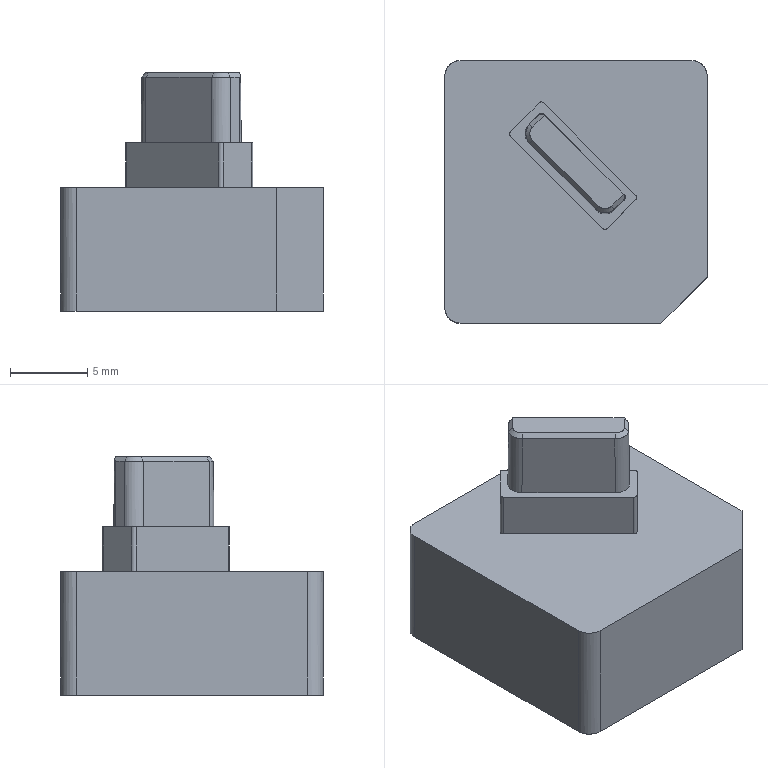NC program | PowerMill | posted with a generic post | part box 17 x 17 x 15.424 mm
Lines 3247 to 4312 of 24748:
N3344 M6
N3345 S18000 M03
N3346 G00 G90 X0.0 Y0.0
N3347 G43 Z10.804 H14
N3348
N3349 G05 P10000 R8
N3350 X1.6082 Y4.7339
N3351 Z0.794
N3352 G01 Z-0.406 F1200.0
N3353 X1.5606 Y4.6806 F2000.0
N3354 X1.5193 Y4.6224
N3355 X1.4846 Y4.5599
N3356 X1.4572 Y4.4939
N3357 X1.4373 Y4.4253
N3358 X1.4251 Y4.3549
N3359 X1.4209 Y4.2836
N3360 X1.4247 Y4.2122
N3361 X1.4363 Y4.1418
N3362 X1.4558 Y4.073
N3363 X1.4828 Y4.0068
N3364 X1.517 Y3.9441
N3365 X1.558 Y3.8856
N3366 X1.6053 Y3.832
N3367 X1.6085 Y3.8288
N3368 X1.7494 Y3.688
N3369 X2.1047 Y3.3323
N3370 X2.4605 Y2.9769
N3371 X3.1826 Y2.2539
N3372 X3.4605 Y1.977
N3373 X3.7378 Y1.6995
N3374 X3.8898 Y1.5451
N3375 X4.0697 Y1.3685
N3376 X4.1747 Y1.2654
N3377 X4.3095 Y1.1279
N3378 X4.4178 Y1.0089
N3379 X4.4892 Y0.9237
N3380 X4.5558 Y0.8347
N3381 X4.6169 Y0.7398
N3382 X4.6724 Y0.6391
N3383 X4.7218 Y0.5327
N3384 X4.7651 Y0.4211
N3385 X4.8017 Y0.3045
N3386 X4.83 Y0.1893
N3387 X4.8506 Y0.0727
N3388 X4.8634 Y-0.045
N3389 X4.8684 Y-0.1635
N3390 X4.8654 Y-0.2822
N3391 X4.8545 Y-0.4008
N3392 X4.8356 Y-0.5187
N3393 X4.8089 Y-0.6353
N3394 X4.7743 Y-0.7501
N3395 X4.7322 Y-0.8625
N3396 X4.6826 Y-0.9719
N3397 X4.626 Y-1.0778
N3398 X4.5624 Y-1.1796
N3399 X4.4923 Y-1.2771
N3400 X4.4158 Y-1.3697
N3401 X4.3335 Y-1.4572
N3402 X4.2476 Y-1.542
N3403 X3.857 Y-1.9321
N3404 X3.5858 Y-2.2036
N3405 X3.4823 Y-2.301
N3406 X3.3746 Y-2.3916
N3407 X3.2629 Y-2.4752
N3408 X3.1477 Y-2.5516
N3409 X3.0293 Y-2.6206
N3410 X2.9081 Y-2.6822
N3411 X2.7835 Y-2.7367
N3412 X2.6531 Y-2.7853
N3413 X2.5213 Y-2.8259
N3414 X2.3985 Y-2.8564
N3415 X2.2612 Y-2.8826
N3416 X2.1233 Y-2.9007
N3417 X1.9851 Y-2.9109
N3418 X1.847 Y-2.9131
N3419 X1.7088 Y-2.9074
N3420 X1.5711 Y-2.8936
N3421 X1.4344 Y-2.872
N3422 X1.2994 Y-2.8425
N3423 X1.1664 Y-2.8053
N3424 X1.0358 Y-2.7605
N3425 X0.9081 Y-2.7083
N3426 X0.7837 Y-2.649
N3427 X0.6609 Y-2.5821
N3428 X0.5442 Y-2.5096
N3429 X0.4336 Y-2.4318
N3430 X0.3376 Y-2.3557
N3431 X0.2437 Y-2.2724
N3432 X0.1308 Y-2.1629
N3433 X-0.0749 Y-1.9571
N3434 X-1.3805 Y-0.6516
N3435 X-3.5829 Y1.5506
N3436 X-4.0378 Y2.0056
N3437 X-4.1367 Y2.1062
N3438 X-4.2297 Y2.2114
N3439 X-4.3162 Y2.3212
N3440 X-4.396 Y2.4353
N3441 X-4.4689 Y2.5535
N3442 X-4.5347 Y2.6753
N3443 X-4.5933 Y2.8005
N3444 X-4.6445 Y2.9287
N3445 X-4.6881 Y3.0596
N3446 X-4.7241 Y3.1928
N3447 X-4.7524 Y3.328
N3448 X-4.773 Y3.4648
N3449 X-4.7857 Y3.603
N3450 X-4.7906 Y3.7414
N3451 X-4.7876 Y3.8795
N3452 X-4.7768 Y4.0171
N3453 X-4.758 Y4.1538
N3454 X-4.7314 Y4.2892
N3455 X-4.697 Y4.423
N3456 X-4.6549 Y4.5547
N3457 X-4.6052 Y4.6838
N3458 X-4.548 Y4.8102
N3459 X-4.4836 Y4.9331
N3460 X-4.4122 Y5.0523
N3461 X-4.3339 Y5.1674
N3462 X-4.249 Y5.2781
N3463 X-4.1578 Y5.3839
N3464 X-4.0605 Y5.4849
N3465 X-3.5634 Y5.9813
N3466 X-3.3467 Y6.1994
N3467 X-3.2565 Y6.2851
N3468 X-3.1621 Y6.3638
N3469 X-3.064 Y6.4354
N3470 X-2.9625 Y6.4997
N3471 X-2.858 Y6.5566
N3472 X-2.7505 Y6.6062
N3473 X-2.6399 Y6.6485
N3474 X-2.5266 Y6.6833
N3475 X-2.4111 Y6.7107
N3476 X-2.2939 Y6.7302
N3477 X-2.1753 Y6.742
N3478 X-2.0558 Y6.7458
N3479 X-1.9361 Y6.7417
N3480 X-1.8167 Y6.7296
N3481 X-1.698 Y6.7095
N3482 X-1.5807 Y6.6816
N3483 X-1.4655 Y6.6459
N3484 X-1.3528 Y6.6027
N3485 X-1.2432 Y6.5522
N3486 X-1.137 Y6.4946
N3487 X-1.0599 Y6.4468
N3488 X-0.9887 Y6.3962
N3489 X-0.9208 Y6.3415
N3490 X-0.8478 Y6.2777
N3491 X-0.7663 Y6.2019
N3492 X-0.6736 Y6.1117
N3493 X-0.5647 Y6.0027
N3494 X-0.4285 Y5.8654
N3495 X-0.3645 Y5.8013
N3496 X0.0232 Y5.4136
N3497 X0.4112 Y5.0263
N3498 X1.3049 Y4.1322
N3499 X1.6085 Y3.8288
N3500 X1.6617 Y3.7812
N3501 X1.72 Y3.7398
N3502 X1.7825 Y3.7052
N3503 X1.8485 Y3.6777
N3504 X1.9171 Y3.6578
N3505 X1.9875 Y3.6457
N3506 X2.0588 Y3.6415
N3507 X2.1301 Y3.6452
N3508 X2.2006 Y3.6569
N3509 X2.2694 Y3.6764
N3510 X2.3355 Y3.7034
N3511 X2.3983 Y3.7376
N3512 X2.4568 Y3.7786
N3513 X2.5103 Y3.8258
N3514 X2.5136 Y3.8291
N3515 X1.6086 Y4.734 Z-0.426
N3516 X1.561 Y4.6808
N3517 X1.5196 Y4.6226
N3518 X1.485 Y4.5601
N3519 X1.4575 Y4.4941
N3520 X1.4376 Y4.4255
N3521 X1.4254 Y4.3551
N3522 X1.4212 Y4.2838
N3523 X1.4249 Y4.2124
N3524 X1.4366 Y4.1419
N3525 X1.456 Y4.0732
N3526 X1.483 Y4.007
N3527 X1.5172 Y3.9443
N3528 X1.5582 Y3.8858
N3529 X1.6054 Y3.8322
N3530 X1.6086 Y3.8289
N3531 X1.7034 Y3.7341
N3532 X3.1654 Y2.2722
N3533 X4.3253 Y1.1117
N3534 X4.4129 Y1.0183
N3535 X4.4933 Y0.9212
N3536 X4.5663 Y0.8208
N3537 X4.6319 Y0.7172
N3538 X4.6891 Y0.6125
N3539 X4.7392 Y0.5044
N3540 X4.7819 Y0.3931
N3541 X4.8171 Y0.2793
N3542 X4.8447 Y0.1633
N3543 X4.8645 Y0.0455
N3544 X4.8764 Y-0.0736
N3545 X4.8804 Y-0.1933
N3546 X4.8764 Y-0.3132
N3547 X4.8644 Y-0.4324
N3548 X4.8445 Y-0.5505
N3549 X4.8169 Y-0.6669
N3550 X4.7817 Y-0.7811
N3551 X4.739 Y-0.8925
N3552 X4.689 Y-1.0008
N3553 X4.6343 Y-1.1016
N3554 X4.5723 Y-1.1993
N3555 X4.5021 Y-1.2956
N3556 X4.4231 Y-1.3903
N3557 X4.3353 Y-1.4835
N3558 X4.2405 Y-1.5774
N3559 X3.7611 Y-2.0567
N3560 X3.6142 Y-2.2038
N3561 X3.5119 Y-2.3013
N3562 X3.4052 Y-2.3928
N3563 X3.2962 Y-2.4764
N3564 X3.185 Y-2.5518
N3565 X3.0717 Y-2.6197
N3566 X2.9544 Y-2.6818
N3567 X2.828 Y-2.7399
N3568 X2.6983 Y-2.7907
N3569 X2.5657 Y-2.8341
N3570 X2.484 Y-2.8567
N3571 X2.4027 Y-2.8752
N3572 X2.3561 Y-2.8859
N3573 X2.2219 Y-2.9087
N3574 X2.0826 Y-2.9246
N3575 X1.9515 Y-2.9323
N3576 X1.8203 Y-2.9326
N3577 X1.6805 Y-2.9252
N3578 X1.5419 Y-2.9098
N3579 X1.4049 Y-2.8866
N3580 X1.2699 Y-2.8556
N3581 X1.1375 Y-2.8171
N3582 X1.0076 Y-2.7711
N3583 X0.8774 Y-2.7166
N3584 X0.7512 Y-2.6552
N3585 X0.6296 Y-2.5872
N3586 X0.5128 Y-2.5129
N3587 X0.4012 Y-2.4324
N3588 X0.3077 Y-2.357
N3589 X0.2162 Y-2.2744
N3590 X0.1018 Y-2.1623
N3591 X-0.2422 Y-1.8183
N3592 X-3.3461 Y1.2858
N3593 X-4.0838 Y2.0235
N3594 X-4.18 Y2.1239
N3595 X-4.2702 Y2.2292
N3596 X-4.3542 Y2.3392
N3597 X-4.4319 Y2.4539
N3598 X-4.5028 Y2.5728
N3599 X-4.567 Y2.6956
N3600 X-4.624 Y2.8221
N3601 X-4.6737 Y2.9517
N3602 X-4.716 Y3.0841
N3603 X-4.7507 Y3.2188
N3604 X-4.7776 Y3.3555
N3605 X-4.7967 Y3.4935
N3606 X-4.8078 Y3.6324
N3607 X-4.8109 Y3.7716
N3608 X-4.806 Y3.9106
N3609 X-4.7933 Y4.049
N3610 X-4.7726 Y4.1862
N3611 X-4.7441 Y4.322
N3612 X-4.708 Y4.4559
N3613 X-4.6643 Y4.5874
N3614 X-4.6133 Y4.7161
N3615 X-4.5549 Y4.8416
N3616 X-4.4894 Y4.9638
N3617 X-4.4167 Y5.0824
N3618 X-4.337 Y5.1971
N3619 X-4.2505 Y5.3076
N3620 X-4.1573 Y5.4137
N3621 X-4.0583 Y5.5154
N3622 X-3.7646 Y5.8078
N3623 X-3.5421 Y6.031
N3624 X-3.4533 Y6.1222
N3625 X-3.3602 Y6.2152
N3626 X-3.2654 Y6.3024
N3627 X-3.1692 Y6.3821
N3628 X-3.0725 Y6.4529
N3629 X-2.975 Y6.5148
N3630 X-2.8765 Y6.5684
N3631 X-2.7764 Y6.6145
N3632 X-2.6743 Y6.6538
N3633 X-2.5699 Y6.6871
N3634 X-2.4614 Y6.7151
N3635 X-2.3448 Y6.7373
N3636 X-2.2271 Y6.7516
N3637 X-2.1085 Y6.758
N3638 X-1.9895 Y6.7565
N3639 X-1.8706 Y6.7471
N3640 X-1.7523 Y6.7296
N3641 X-1.6353 Y6.7043
N3642 X-1.52 Y6.6712
N3643 X-1.4071 Y6.6305
N3644 X-1.2971 Y6.5823
N3645 X-1.1905 Y6.527
N3646 X-1.0876 Y6.4647
N3647 X-0.9908 Y6.397
N3648 X-0.8943 Y6.3201
N3649 X-0.7953 Y6.2314
N3650 X-0.6911 Y6.1286
N3651 X0.0252 Y5.4123
N3652 X1.6086 Y3.8289
N3653 X1.6619 Y3.7813
N3654 X1.7201 Y3.7399
N3655 X1.7826 Y3.7053
N3656 X1.8486 Y3.6778
N3657 X1.9172 Y3.6579
N3658 X1.9876 Y3.6457
N3659 X2.0589 Y3.6415
N3660 X2.1302 Y3.6452
N3661 X2.2007 Y3.6569
N3662 X2.2694 Y3.6763
N3663 X2.3356 Y3.7033
N3664 X2.3984 Y3.7375
N3665 X2.4569 Y3.7785
N3666 X2.5105 Y3.8257
N3667 X2.5137 Y3.8289
N3668 X1.6088 Y4.7341 Z-0.446
N3669 X1.5611 Y4.6809
N3670 X1.5198 Y4.6227
N3671 X1.4851 Y4.5602
N3672 X1.4576 Y4.4942
N3673 X1.4377 Y4.4256
N3674 X1.4255 Y4.3552
N3675 X1.4213 Y4.2839
N3676 X1.425 Y4.2125
N3677 X1.4367 Y4.1421
N3678 X1.4561 Y4.0733
N3679 X1.4831 Y4.0071
N3680 X1.5173 Y3.9444
N3681 X1.5583 Y3.8859
N3682 X1.6055 Y3.8323
N3683 X1.6087 Y3.8291
N3684 X2.0613 Y3.3764
N3685 X4.1939 Y1.244
N3686 X4.3256 Y1.1122
N3687 X4.4086 Y1.024
N3688 X4.4869 Y0.9299
N3689 X4.5609 Y0.8286
N3690 X4.6298 Y0.7212
N3691 X4.6883 Y0.6175
N3692 X4.7399 Y0.5102
N3693 X4.7841 Y0.3997
N3694 X4.821 Y0.2865
N3695 X4.8502 Y0.1709
N3696 X4.8717 Y0.0533
N3697 X4.8853 Y-0.0657
N3698 X4.891 Y-0.1855
N3699 X4.8887 Y-0.3054
N3700 X4.8785 Y-0.4249
N3701 X4.8603 Y-0.5435
N3702 X4.8343 Y-0.6607
N3703 X4.8017 Y-0.7729
N3704 X4.7617 Y-0.8824
N3705 X4.7142 Y-0.9896
N3706 X4.6592 Y-1.0942
N3707 X4.5966 Y-1.1962
N3708 X4.5264 Y-1.2955
N3709 X4.4485 Y-1.3918
N3710 X4.3629 Y-1.4851
N3711 X4.2708 Y-1.576
N3712 X3.9386 Y-1.9067
N3713 X3.6429 Y-2.2042
N3714 X3.5336 Y-2.3086
N3715 X3.423 Y-2.4037
N3716 X3.311 Y-2.49
N3717 X3.1978 Y-2.5675
N3718 X3.0833 Y-2.6366
N3719 X2.9671 Y-2.6978
N3720 X2.835 Y-2.7584
N3721 X2.7066 Y-2.8091
N3722 X2.5809 Y-2.8507
N3723 X2.5601 Y-2.8568
N3724 X2.4254 Y-2.8915
N3725 X2.4067 Y-2.8952
N3726 X2.2878 Y-2.9187
N3727 X2.1481 Y-2.9381
N3728 X2.0076 Y-2.9496
N3729 X1.8672 Y-2.9532
N3730 X1.7279 Y-2.9488
N3731 X1.5906 Y-2.9365
N3732 X1.4547 Y-2.9165
N3733 X1.3183 Y-2.8883
N3734 X1.1828 Y-2.8522
N3735 X1.0491 Y-2.8083
N3736 X0.9185 Y-2.757
N3737 X0.7916 Y-2.6986
N3738 X0.6693 Y-2.6337
N3739 X0.5522 Y-2.5626
N3740 X0.4588 Y-2.499
N3741 X0.3682 Y-2.4316
N3742 X0.2811 Y-2.3598
N3743 X0.1975 Y-2.2838
N3744 X0.1164 Y-2.205
N3745 X0.0365 Y-2.1252
N3746 X-1.7839 Y-0.3048
N3747 X-3.5094 Y1.4207
N3748 X-4.0256 Y1.9372
N3749 X-4.1284 Y2.0408
N3750 X-4.2228 Y2.1419
N3751 X-4.3112 Y2.2484
N3752 X-4.3937 Y2.3601
N3753 X-4.4698 Y2.4766
N3754 X-4.5393 Y2.5976
N3755 X-4.6019 Y2.7227
N3756 X-4.6572 Y2.8511
N3757 X-4.7055 Y2.9833
N3758 X-4.7461 Y3.1176
N3759 X-4.7788 Y3.2536
N3760 X-4.8037 Y3.3909
N3761 X-4.8206 Y3.529
N3762 X-4.8296 Y3.6678
N3763 X-4.8306 Y3.8067
N3764 X-4.8236 Y3.9454
N3765 X-4.8088 Y4.0837
N3766 X-4.786 Y4.2225
N3767 X-4.7554 Y4.3593
N3768 X-4.7172 Y4.4939
N3769 X-4.6715 Y4.6258
N3770 X-4.6184 Y4.7546
N3771 X-4.558 Y4.8801
N3772 X-4.4906 Y5.0018
N3773 X-4.4163 Y5.1195
N3774 X-4.3353 Y5.2329
N3775 X-4.2478 Y5.3417
N3776 X-4.1541 Y5.4456
N3777 X-4.0557 Y5.5461
N3778 X-3.7666 Y5.8346
N3779 X-3.5192 Y6.0827
N3780 X-3.4392 Y6.1642
N3781 X-3.3578 Y6.2444
N3782 X-3.2691 Y6.3259
N3783 X-3.1772 Y6.4018
N3784 X-3.0898 Y6.4651
N3785 X-3.005 Y6.5186
N3786 X-2.9195 Y6.5658
N3787 X-2.8314 Y6.6083
N3788 X-2.741 Y6.6464
N3789 X-2.6281 Y6.6861
N3790 X-2.5126 Y6.7183
N3791 X-2.3952 Y6.7428
N3792 X-2.2764 Y6.7594
N3793 X-2.1569 Y6.768
N3794 X-2.0374 Y6.7687
N3795 X-1.9185 Y6.7614
N3796 X-1.8008 Y6.7462
N3797 X-1.6848 Y6.7233
N3798 X-1.571 Y6.6927
N3799 X-1.4596 Y6.6545
N3800 X-1.3677 Y6.6166
N3801 X-1.2804 Y6.5757
N3802 X-1.1951 Y6.5308
N3803 X-1.1106 Y6.4807
N3804 X-1.0251 Y6.4231
N3805 X-0.9359 Y6.355
N3806 X-0.8393 Y6.2719
N3807 X-0.7449 Y6.1828
N3808 X-0.6599 Y6.0984
N3809 X-0.58 Y6.0174
N3810 X-0.502 Y5.9386
N3811 X-0.4241 Y5.861
N3812 X-0.3431 Y5.7812
N3813 X-0.0454 Y5.4831
N3814 X0.268 Y5.1701
N3815 X0.7299 Y4.7077
N3816 X1.1885 Y4.2493
N3817 X1.6087 Y3.8291
N3818 X1.662 Y3.7814
N3819 X1.7202 Y3.7401
N3820 X1.7827 Y3.7054
N3821 X1.8487 Y3.6779
N3822 X1.9173 Y3.658
N3823 X1.9877 Y3.6458
N3824 X2.059 Y3.6416
N3825 X2.1303 Y3.6453
N3826 X2.2008 Y3.657
N3827 X2.2696 Y3.6764
N3828 X2.3358 Y3.7034
N3829 X2.3985 Y3.7376
N3830 X2.457 Y3.7786
N3831 X2.5106 Y3.8258
N3832 X2.5138 Y3.829
N3833 X1.6088 Y4.7343 Z-0.466
N3834 X1.5612 Y4.681
N3835 X1.5198 Y4.6228
N3836 X1.4852 Y4.5603
N3837 X1.4577 Y4.4943
N3838 X1.4378 Y4.4257
N3839 X1.4256 Y4.3553
N3840 X1.4214 Y4.284
N3841 X1.4251 Y4.2126
N3842 X1.4368 Y4.1422
N3843 X1.4562 Y4.0734
N3844 X1.4832 Y4.0072
N3845 X1.5174 Y3.9445
N3846 X1.5584 Y3.886
N3847 X1.6056 Y3.8324
N3848 X1.6088 Y3.8292
N3849 X2.0042 Y3.4339
N3850 X3.2344 Y2.2035
N3851 X4.3256 Y1.1125
N3852 X4.4075 Y1.0257
N3853 X4.485 Y0.9333
N3854 X4.558 Y0.8343
N3855 X4.6262 Y0.7283
N3856 X4.6884 Y0.6181
N3857 X4.7412 Y0.5113
N3858 X4.787 Y0.4014
N3859 X4.8253 Y0.2886
N3860 X4.856 Y0.1735
N3861 X4.879 Y0.0563
N3862 X4.8941 Y-0.0623
N3863 X4.9013 Y-0.1817
N3864 X4.9005 Y-0.3012
N3865 X4.8917 Y-0.4203
N3866 X4.8751 Y-0.5383
N3867 X4.8506 Y-0.6549
N3868 X4.8184 Y-0.7696
N3869 X4.7789 Y-0.8819
N3870 X4.7318 Y-0.9927
N3871 X4.6787 Y-1.0979
N3872 X4.6199 Y-1.197
N3873 X4.556 Y-1.2898
N3874 X4.487 Y-1.3761
N3875 X4.413 Y-1.458
N3876 X4.3319 Y-1.5427
N3877 X4.2496 Y-1.6263
N3878 X4.1622 Y-1.7138
N3879 X4.0383 Y-1.8366
N3880 X3.9548 Y-1.919
N3881 X3.8713 Y-2.0016
N3882 X3.7881 Y-2.0844
N3883 X3.7056 Y-2.1678
N3884 X3.6234 Y-2.2517
N3885 X3.5186 Y-2.3498
N3886 X3.4097 Y-2.4408
N3887 X3.2974 Y-2.5245
N3888 X3.1807 Y-2.6017
N3889 X3.0591 Y-2.6725
N3890 X2.934 Y-2.7362
N3891 X2.806 Y-2.7925
N3892 X2.6754 Y-2.8412
N3893 X2.6286 Y-2.8565
N3894 X2.4933 Y-2.8954
N3895 X2.411 Y-2.9141
N3896 X2.3561 Y-2.9266
N3897 X2.2176 Y-2.9499
N3898 X2.0781 Y-2.9652
N3899 X1.938 Y-2.9726
N3900 X1.7979 Y-2.972
N3901 X1.6582 Y-2.9634
N3902 X1.5193 Y-2.9469
N3903 X1.3815 Y-2.9225
N3904 X1.2452 Y-2.8903
N3905 X1.1107 Y-2.8504
N3906 X0.9781 Y-2.8028
N3907 X0.8483 Y-2.7476
N3908 X0.722 Y-2.6853
N3909 X0.5996 Y-2.616
N3910 X0.4813 Y-2.5399
N3911 X0.3798 Y-2.4666
N3912 X0.2803 Y-2.3855
N3913 X0.1735 Y-2.289
N3914 X0.0813 Y-2.199
N3915 X-1.4919 Y-0.6251
N3916 X-2.6883 Y0.5713
N3917 X-3.6907 Y1.5736
N3918 X-3.9949 Y1.8764
N3919 X-4.0877 Y1.9693
N3920 X-4.2017 Y2.0889
N3921 X-4.2928 Y2.1931
N3922 X-4.3727 Y2.2955
N3923 X-4.4479 Y2.4046
N3924 X-4.5197 Y2.5225
N3925 X-4.5882 Y2.6501
N3926 X-4.6465 Y2.7732
N3927 X-4.6978 Y2.9
N3928 X-4.7421 Y3.0307
N3929 X-4.7792 Y3.1649
N3930 X-4.8088 Y3.3021
N3931 X-4.8308 Y3.4412
N3932 X-4.8448 Y3.5808
N3933 X-4.8509 Y3.7208
N3934 X-4.849 Y3.8607
N3935 X-4.8391 Y4.0002
N3936 X-4.8212 Y4.1391
N3937 X-4.7954 Y4.2769
N3938 X-4.7618 Y4.4133
N3939 X-4.7204 Y4.5479
N3940 X-4.6713 Y4.6805
N3941 X-4.6153 Y4.809
N3942 X-4.5522 Y4.9338
N3943 X-4.4823 Y5.0545
N3944 X-4.4058 Y5.1706
N3945 X-4.3231 Y5.2817
N3946 X-4.2345 Y5.3875
N3947 X-4.1401 Y5.4879
N3948 X-3.8296 Y5.8006
N3949 X-3.6717 Y5.9561
N3950 X-3.5532 Y6.0759
N3951 X-3.421 Y6.2112
N3952 X-3.3213 Y6.3067
N3953 X-3.2327 Y6.3832
N3954 X-3.1454 Y6.4493
N3955 X-3.0451 Y6.5154
N3956 X-2.9411 Y6.5744
N3957 X-2.834 Y6.6261
N3958 X-2.7242 Y6.6703
N3959 X-2.6117 Y6.7071
N3960 X-2.4952 Y6.7369
N3961 X-2.3769 Y6.759
N3962 X-2.2575 Y6.7731
N3963 X-2.1375 Y6.7793
N3964 X-2.0177 Y6.7775
N3965 X-1.8987 Y6.7677
N3966 X-1.7809 Y6.7501
N3967 X-1.665 Y6.7248
N3968 X-1.5514 Y6.6918
N3969 X-1.4404 Y6.6513
N3970 X-1.3478 Y6.6108
N3971 X-1.2602 Y6.5673
N3972 X-1.1748 Y6.5202
N3973 X-1.0919 Y6.4693
N3974 X-1.0116 Y6.4142
N3975 X-0.9334 Y6.3544
N3976 X-0.8531 Y6.2862
N3977 X-0.7651 Y6.2041
N3978 X-0.6505 Y6.0894
N3979 X-0.5713 Y6.0094
N3980 X0.6244 Y4.8135
N3981 X1.6088 Y3.8292
N3982 X1.6621 Y3.7815
N3983 X1.7203 Y3.7402
N3984 X1.7828 Y3.7055
N3985 X1.8488 Y3.6781
N3986 X1.9174 Y3.6581
N3987 X1.9878 Y3.646
N3988 X2.0591 Y3.6417
N3989 X2.1305 Y3.6455
N3990 X2.2009 Y3.6571
N3991 X2.2697 Y3.6766
N3992 X2.3359 Y3.7036
N3993 X2.3986 Y3.7378
N3994 X2.4571 Y3.7788
N3995 X2.5107 Y3.826
N3996 X2.5139 Y3.8292
N3997 X1.609 Y4.7344 Z-0.486
N3998 X1.5614 Y4.6812
N3999 X1.52 Y4.6229
N4000 X1.4854 Y4.5605
N4001 X1.4579 Y4.4944
N4002 X1.4379 Y4.4258
N4003 X1.4258 Y4.3554
N4004 X1.4216 Y4.2841
N4005 X1.4253 Y4.2128
N4006 X1.4369 Y4.1423
N4007 X1.4564 Y4.0736
N4008 X1.4834 Y4.0074
N4009 X1.5176 Y3.9447
N4010 X1.5586 Y3.8861
N4011 X1.6058 Y3.8326
N4012 X1.609 Y3.8293
N4013 X1.9336 Y3.5047
N4014 X3.9286 Y1.51
N4015 X4.3256 Y1.1127
N4016 X4.4124 Y1.0202
N4017 X4.4935 Y0.922
N4018 X4.5688 Y0.8185
N4019 X4.6378 Y0.71
N4020 X4.7004 Y0.5968
N4021 X4.7561 Y0.4794
N4022 X4.8008 Y0.3689
N4023 X4.8382 Y0.2558
N4024 X4.868 Y0.1406
N4025 X4.8901 Y0.0236
N4026 X4.9043 Y-0.0946
N4027 X4.9106 Y-0.2137
N4028 X4.909 Y-0.3333
N4029 X4.8994 Y-0.4526
N4030 X4.8819 Y-0.5711
N4031 X4.8565 Y-0.6883
N4032 X4.8234 Y-0.8034
N4033 X4.7827 Y-0.9159
N4034 X4.7347 Y-1.0254
N4035 X4.6796 Y-1.1313
N4036 X4.6176 Y-1.2333
N4037 X4.5491 Y-1.3309
N4038 X4.4851 Y-1.4109
N4039 X4.4126 Y-1.4905
N4040 X4.3146 Y-1.588
N4041 X4.2022 Y-1.6981
N4042 X4.1 Y-1.8019
N4043 X3.8189 Y-2.0824
N4044 X3.6726 Y-2.2299
N4045 X3.5662 Y-2.3333
N4046 X3.4608 Y-2.4255
N4047 X3.3559 Y-2.5074
N4048 X3.2469 Y-2.5832
N4049 X3.126 Y-2.6578
N4050 X3.0018 Y-2.7252
N4051 X2.8749 Y-2.7851
N4052 X2.7458 Y-2.8372
N4053 X2.6921 Y-2.8564
N4054 X2.5575 Y-2.8986
N4055 X2.4208 Y-2.9332
N4056 X2.4149 Y-2.9344
N4057 X2.2823 Y-2.9601
N4058 X2.1425 Y-2.979
N4059 X2.0018 Y-2.9901
N4060 X1.8608 Y-2.9932
N4061 X1.7199 Y-2.9883
N4062 X1.5797 Y-2.9754
N4063 X1.4407 Y-2.9547
N4064 X1.3033 Y-2.9261
N4065 X1.168 Y-2.8899
N4066 X1.0351 Y-2.846
N4067 X0.9049 Y-2.7946
N4068 X0.7778 Y-2.7359
N4069 X0.688 Y-2.6889
N4070 X0.5999 Y-2.6388
N4071 X0.5139 Y-2.5858
N4072 X0.4301 Y-2.5294
N4073 X0.349 Y-2.4692
N4074 X0.2699 Y-2.4046
N4075 X0.1806 Y-2.3242
N4076 X0.0809 Y-2.2272
N4077 X0.001 Y-2.1467
N4078 X-0.0707 Y-2.0746
N4079 X-0.1456 Y-2.0
N4080 X-0.7117 Y-1.4333
N4081 X-1.2984 Y-0.8469
N4082 X-2.4609 Y0.3154
N4083 X-3.5327 Y1.3874
N4084 X-3.8994 Y1.7541
N4085 X-4.0233 Y1.8763
N4086 X-4.1526 Y2.0071
N4087 X-4.2596 Y2.1243
N4088 X-4.3507 Y2.2341
N4089 X-4.4292 Y2.3398
N4090 X-4.4975 Y2.4441
N4091 X-4.5691 Y2.5683
N4092 X-4.6335 Y2.6958
N4093 X-4.6903 Y2.8262
N4094 X-4.7396 Y2.9592
N4095 X-4.7812 Y3.0942
N4096 X-4.8149 Y3.2304
N4097 X-4.8408 Y3.3679
N4098 X-4.8588 Y3.5067
N4099 X-4.8689 Y3.6464
N4100 X-4.8711 Y3.7868
N4101 X-4.8652 Y3.9274
N4102 X-4.8514 Y4.068
N4103 X-4.8296 Y4.2083
N4104 X-4.8008 Y4.3437
N4105 X-4.764 Y4.4782
N4106 X-4.7193 Y4.612
N4107 X-4.6667 Y4.7437
N4108 X-4.6071 Y4.8718
N4109 X-4.541 Y4.9952
N4110 X-4.4759 Y5.1021
N4111 X-4.4056 Y5.2055
N4112 X-4.33 Y5.3051
N4113 X-4.2429 Y5.4081
N4114 X-4.1434 Y5.5151
N4115 X-4.0507 Y5.6086
N4116 X-3.9562 Y5.7016
N4117 X-3.7006 Y5.9575
N4118 X-3.4451 Y6.2137
N4119 X-3.3615 Y6.2961
N4120 X-3.2745 Y6.3742
N4121 X-3.1824 Y6.4463
N4122 X-3.0852 Y6.5124
N4123 X-2.9831 Y6.5721
N4124 X-2.8767 Y6.6251
N4125 X-2.7664 Y6.6711
N4126 X-2.6527 Y6.7099
N4127 X-2.5361 Y6.7412
N4128 X-2.4173 Y6.7649
N4129 X-2.3011 Y6.7803
N4130 X-2.1849 Y6.788
N4131 X-2.0684
N4132 X-1.9518 Y6.7803
N4133 X-1.8352 Y6.7648
N4134 X-1.7188 Y6.7414
N4135 X-1.603 Y6.71
N4136 X-1.4879 Y6.6707
N4137 X-1.3739 Y6.6233
N4138 X-1.2614 Y6.568
N4139 X-1.1508 Y6.5048
N4140 X-1.0425 Y6.4338
N4141 X-0.9372 Y6.3552
N4142 X-0.8352 Y6.2693
N4143 X-0.7374 Y6.1764
N4144 X-0.6414 Y6.0796
N4145 X-0.1617 Y5.6003
N4146 X0.3766 Y5.0617
N4147 X1.609 Y3.8293
N4148 X1.6623 Y3.7817
N4149 X1.7205 Y3.7403
N4150 X1.783 Y3.7057
N4151 X1.849 Y3.6782
N4152 X1.9176 Y3.6583
N4153 X1.988 Y3.6461
N4154 X2.0593 Y3.6419
N4155 X2.1306 Y3.6456
N4156 X2.2011 Y3.6573
N4157 X2.2698 Y3.6767
N4158 X2.336 Y3.7037
N4159 X2.3988 Y3.7379
N4160 X2.4573 Y3.7789
N4161 X2.5109 Y3.8261
N4162 X2.5141 Y3.8293
N4163 X1.6091 Y4.7345 Z-0.506
N4164 X1.5614 Y4.6813
N4165 X1.5201 Y4.623
N4166 X1.4854 Y4.5605
N4167 X1.4579 Y4.4945
N4168 X1.438 Y4.4259
N4169 X1.4259 Y4.3555
N4170 X1.4216 Y4.2842
N4171 X1.4254 Y4.2129
N4172 X1.437 Y4.1424
N4173 X1.4565 Y4.0737
N4174 X1.4835 Y4.0075
N4175 X1.5177 Y3.9447
N4176 X1.5587 Y3.8862
N4177 X1.6059 Y3.8327
N4178 X1.6091 Y3.8294
N4179 X2.2857 Y3.1529
N4180 X3.3982 Y2.0404
N4181 X4.1622 Y1.2761
N4182 X4.3062 Y1.1324
N4183 X4.4013 Y1.0323
N4184 X4.4741 Y0.9475
N4185 X4.5416 Y0.8584
N4186 X4.611 Y0.7541
N4187 X4.6753 Y0.6433
N4188 X4.7343 Y0.526
N4189 X4.7877 Y0.4022
N4190 X4.8283 Y0.2921
N4191 X4.8618 Y0.1797
N4192 X4.8877 Y0.0649
N4193 X4.9059 Y-0.0521
N4194 X4.9163 Y-0.1706
N4195 X4.9189 Y-0.2901
N4196 X4.9134 Y-0.41
N4197 X4.8999 Y-0.5298
N4198 X4.8785 Y-0.6486
N4199 X4.8502 Y-0.7627
N4200 X4.8143 Y-0.8749
N4201 X4.7706 Y-0.9853
N4202 X4.7192 Y-1.0935
N4203 X4.6603 Y-1.1988
N4204 X4.6022 Y-1.2885
N4205 X4.535 Y-1.378
N4206 X4.4558 Y-1.4708
N4207 X4.3612 Y-1.5701
N4208 X4.2457 Y-1.6841
N4209 X4.0349 Y-1.8967
N4210 X3.8508 Y-2.0797
N4211 X3.673 Y-2.2585
N4212 X3.5697 Y-2.3574
N4213 X3.4602 Y-2.4513
N4214 X3.3489 Y-2.5367
N4215 X3.2331 Y-2.616
N4216 X3.1127 Y-2.6887
N4217 X2.988 Y-2.7546
N4218 X2.8598 Y-2.8134
N4219 X2.7514 Y-2.8564
N4220 X2.6165 Y-2.9022
N4221 X2.4796 Y-2.9401
N4222 X2.419 Y-2.9533
N4223 X2.3414 Y-2.9702
N4224 X2.202 Y-2.9924
N4225 X2.0615 Y-3.0067
N4226 X1.9205 Y-3.013
N4227 X1.7793 Y-3.0114
N4228 X1.6384 Y-3.0018
N4229 X1.498 Y-2.9843
N4230 X1.3588 Y-2.9588
N4231 X1.2211 Y-2.9255
N4232 X1.0855 Y-2.8846
N4233 X0.9526 Y-2.836
N4234 X0.8227 Y-2.7802
N4235 X0.6964 Y-2.7171
N4236 X0.5739 Y-2.6471
N4237 X0.4556 Y-2.5703
N4238 X0.3417 Y-2.4869
N4239 X0.2328 Y-2.3972
N4240 X0.1288 Y-2.3017
N4241 X0.0013 Y-2.1754
N4242 X-0.1899 Y-1.9837
N4243 X-2.5486 Y0.375
N4244 X-3.5574 Y1.3835
N4245 X-3.8359 Y1.6623
N4246 X-3.8972 Y1.7236
N4247 X-3.9587 Y1.7847
N4248 X-4.0204 Y1.8458
N4249 X-4.0821 Y1.9068
N4250 X-4.1435 Y1.9682
N4251 X-4.2039 Y2.0304
N4252 X-4.2625 Y2.0942
N4253 X-4.3184 Y2.1602
N4254 X-4.3714 Y2.2286
N4255 X-4.4221 Y2.2987
N4256 X-4.4713 Y2.37
N4257 X-4.5442 Y2.4845
N4258 X-4.6108 Y2.604
N4259 X-4.671 Y2.7283
N4260 X-4.7246 Y2.8571
N4261 X-4.7712 Y2.99
N4262 X-4.8107 Y3.1267
N4263 X-4.8423 Y3.2644
N4264 X-4.8662 Y3.4038
N4265 X-4.8821 Y3.5443
N4266 X-4.8901 Y3.6854
N4267 Y3.8269
N4268 X-4.8822 Y3.9681
N4269 X-4.8662 Y4.1086
N4270 X-4.8424 Y4.248
N4271 X-4.8107 Y4.3858
N4272 X-4.7714 Y4.5213
N4273 X-4.7241 Y4.6556
N4274 X-4.6697 Y4.7866
N4275 X-4.6081 Y4.9138
N4276 X-4.5396 Y5.037
N4277 X-4.4644 Y5.156
N4278 X-4.3825 Y5.2705
N4279 X-4.2942 Y5.3803
N4280 X-4.1996 Y5.4852
N4281 X-4.1012 Y5.5848
N4282 X-3.4034 Y6.2834
N4283 X-3.319 Y6.3623
N4284 X-3.229 Y6.4354
N4285 X-3.1336 Y6.5028
N4286 X-3.033 Y6.5641
N4287 X-2.9277 Y6.6189
N4288 X-2.8182 Y6.667
N4289 X-2.705 Y6.7079
N4290 X-2.5886 Y6.7416
N4291 X-2.4698 Y6.7676
N4292 X-2.3543 Y6.785
N4293 X-2.2372 Y6.7947
N4294 X-2.1187 Y6.7965
N4295 X-1.9992 Y6.7904
N4296 X-1.8795 Y6.7763
N4297 X-1.7625 Y6.7546
N4298 X-1.6453 Y6.7247
N4299 X-1.5283 Y6.6867
N4300 X-1.412 Y6.6406
N4301 X-1.297 Y6.5865
N4302 X-1.1838 Y6.5244
N4303 X-1.0732 Y6.4546
N4304 X-0.9657 Y6.3775
N4305 X-0.8622 Y6.2933
N4306 X-0.7632 Y6.2025
N4307 X-0.6682 Y6.1072
N4308 X-0.0741 Y5.5127
N4309 X0.6501 Y4.7883
N4310 X1.6091 Y3.8294
N4311 X1.6624 Y3.7818
N4312 X1.7206 Y3.7404
N4313 X1.7831 Y3.7058
N4314 X1.8491 Y3.6783
N4315 X1.9177 Y3.6584
N4316 X1.9881 Y3.6462
N4317 X2.0594 Y3.642
N4318 X2.1307 Y3.6457
N4319 X2.2012 Y3.6574
N4320 X2.2699 Y3.6768
N4321 X2.3361 Y3.7039
N4322 X2.3989 Y3.738
N4323 X2.4574 Y3.779
N4324 X2.511 Y3.8263
N4325 X2.5142 Y3.8295
N4326 X1.6093 Y4.7347 Z-0.526
N4327 X1.5616 Y4.6814
N4328 X1.5203 Y4.6232
N4329 X1.4856 Y4.5607
N4330 X1.4581 Y4.4947
N4331 X1.4382 Y4.4261
N4332 X1.426 Y4.3557
N4333 X1.4218 Y4.2844
N4334 X1.4255 Y4.2131
N4335 X1.4372 Y4.1426
N4336 X1.4566 Y4.0738
N4337 X1.4836 Y4.0076
N4338 X1.5178 Y3.9449
N4339 X1.5588 Y3.8864
N4340 X1.606 Y3.8328
N4341 X1.6093 Y3.8296
N4342 X3.3262 Y2.1126
N4343 X3.8882 Y1.5507
N4344 X4.3253 Y1.113
N4345 X4.4134 Y1.0187
N4346 X4.4956 Y0.919
N4347 X4.5717 Y0.8142
N4348 X4.6412 Y0.7048
N4349 X4.7037 Y0.5916
N4350 X4.7589 Y0.4751
N4351 X4.8066 Y0.3559
N4352 X4.8467 Y0.2345
N4353 X4.8789 Y0.1115
N4354 X4.902 Y-0.0063
N4355 X4.9172 Y-0.1251
N4356 X4.9245 Y-0.2447
N4357 X4.9238 Y-0.3644
N4358 X4.9151 Y-0.4836
N4359 X4.8985 Y-0.6018
N4360 X4.8741 Y-0.7185
N4361 X4.8419 Y-0.8334
N4362 X4.8022 Y-0.9457
N4363 X4.7566 Y-1.053
N4364 X4.7067 Y-1.1515
N4365 X4.6524 Y-1.2421
N4366 X4.6037 Y-1.3154
N4367 X4.5529 Y-1.3872
N4368 X4.4985 Y-1.4562
N4369 X4.439 Y-1.5213
N4370 X4.3764 Y-1.5835
N4371 X4.3136 Y-1.6454
N4372 X3.9991 Y-1.96
N4373 X3.6727 Y-2.2865
N4374 X3.5688 Y-2.3852
N4375 X3.4598 Y-2.4777
N4376 X3.3463 Y-2.5635
N4377 X3.2284 Y-2.6427
N4378 X3.1067 Y-2.7149
N4379 X2.9813 Y-2.78
N4380 X2.8525 Y-2.8382
N4381 X2.7214 Y-2.8888
N4382 X2.5879 Y-2.9319
N4383 X2.452 Y-2.9674
N4384 X2.423 Y-2.9732
N4385 X2.3136 Y-2.9953
N4386 X2.1725 Y-3.0156
N4387 X2.1405 Y-3.0191
N4388 X1.997 Y-3.0299
N4389 X1.8538 Y-3.0328
N4390 X1.7114 Y-3.0277
N4391 X1.5703 Y-3.0147
N4392 X1.4309 Y-2.9938
N4393 X1.2939 Y-2.9654
N4394 X1.1595 Y-2.9294
N4395 X1.0282 Y-2.886
N4396 X0.9 Y-2.8353
N4397 X0.7749 Y-2.7782
N4398 X0.6455 Y-2.7112
N4399 X0.5244 Y-2.6399
N4400 X0.4109 Y-2.5643
N4401 X0.313 Y-2.4908
N4402 X0.2137 Y-2.4069
N4403 X0.1023 Y-2.3032
N4404 X-0.0414 Y-2.1608
N4405 X-0.2955 Y-1.9064
N4406 X-3.0197 Y0.8179
N4407 X-3.9991 Y1.7972
N4408 X-4.0704 Y1.8681
N4409 X-4.1417 Y1.9391